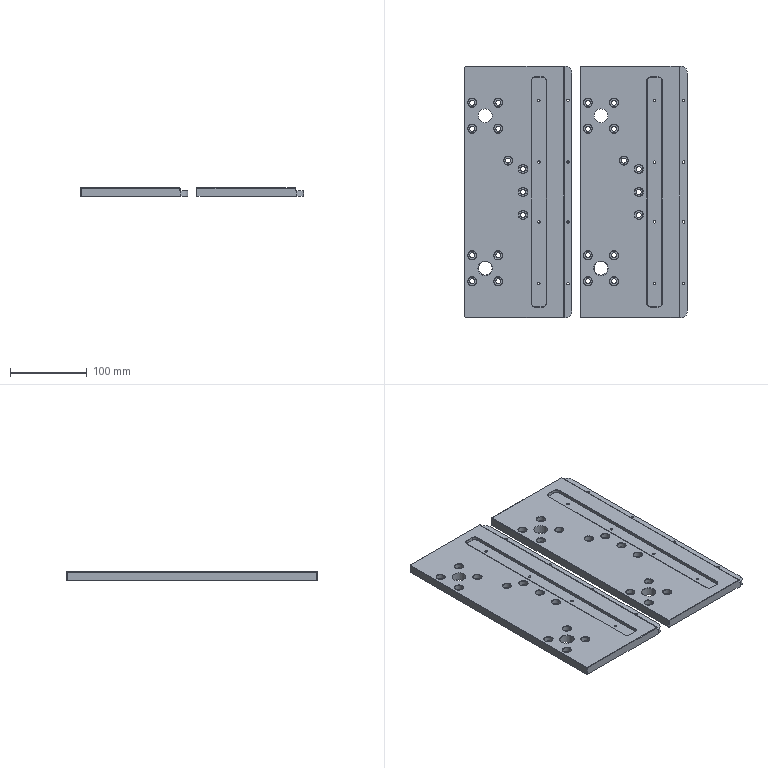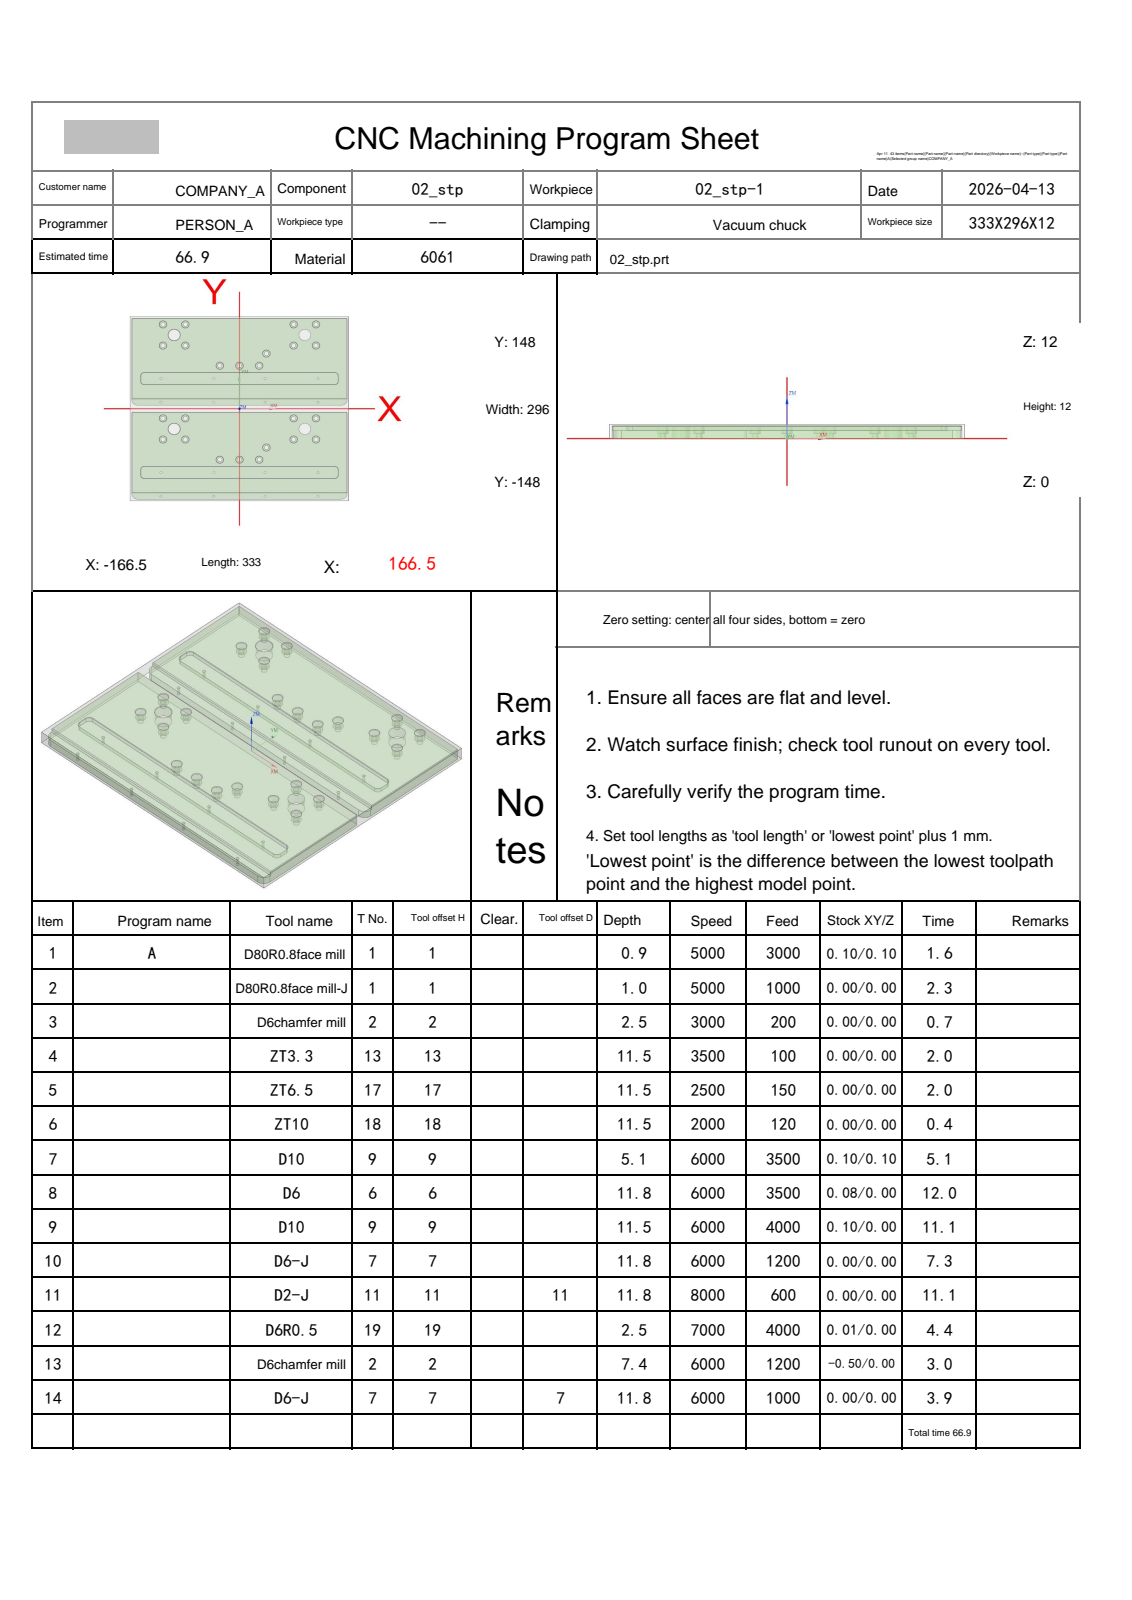NC program | NX | posted by the shop | part box 291 x 328 x 11 mm
Lines 1 to 615 of 9762:
%
O0001
(Machine time: 69.04 MIN)
(===Total Tool:10===)
(T1=D80R0.8 face mill D=80.  R=0.8  D-  H01 Z=11.   )
(T2=D6 chamfer mill   D=6.   R=0.   D-  H02 Z=4.65  )
(T13=ZT3.3  D=3.3  DR_a=118 D-  H13 Z=0.5   )
(T17=ZT6.5  D=6.5  DR_a=118 D-  H17 Z=0.5   )
(T18=ZT10   D=10.  DR_a=118 D-  H18 Z=0.5   )
(T9=D10     D=10.  R=0.   D-  H09 Z=0.5   )
(T6=D6      D=6.   R=0.   D6  H06 Z=0.2   )
(T7=D6-J    D=6.   R=0.   D7  H07 Z=0.2   )
(T11=D2-J   D=2.   R=0.   D11 H11 Z=0.2   )
(T19=D6R0.5 D=6.   R=0.5  D-  H19 Z=9.5   )
G80 G90 G17 G49 G40
G91 G28 Z0
M01
N1 T01 M06
(D80R0.8 face mill  D=80. R=0.8 H=01 ce=0.10 di=0.10)
G00 G90 G54 X-216.097 Y120.945 M03 S5000
G43 H01 Z31.
M08
Z13.55
G01 Z11.55 F3000.
X-204.097 Y121.092
X196.813 Y126.004
X196.897
G02 X204.097 Y118.808 I0.0 J-7.2
G01 Y74.06
G02 X196.199 Y66.065 I-8. J.004
G01 X-196.199 Y61.257
G03 X-204.097 Y53.262 I.102 J-7.999
G01 Y8.514
G03 X-196.897 Y1.317 I7.2 J.004
G01 X-196.813 Y1.318
X196.813 Y6.14
X196.897 Y6.141
G02 X204.097 Y-1.055 I0.0 J-7.2
G01 Y-6.5
Y-45.803
G02 X196.199 Y-53.799 I-8. J.004
G01 X-196.199 Y-58.606
G03 X-204.097 Y-66.602 I.102 J-7.999
G01 Y-111.349
G03 X-196.897 Y-118.546 I7.2 J.004
G01 X-196.813 Y-118.545
X204.097 Y-113.633
X216.097 Y-113.486
Z13.55
G00 X-216.097 Y120.945
Z13.1
G01 Z11.1
X-204.097 Y121.092
X196.813 Y126.004
X196.897
G02 X204.097 Y118.808 I0.0 J-7.2
G01 Y74.06
G02 X196.199 Y66.065 I-8. J.004
G01 X-196.199 Y61.257
G03 X-204.097 Y53.262 I.102 J-7.999
G01 Y8.514
G03 X-196.897 Y1.317 I7.2 J.004
G01 X-196.813 Y1.318
X196.813 Y6.14
X196.897 Y6.141
G02 X204.097 Y-1.055 I0.0 J-7.2
G01 Y-6.5
Y-45.803
G02 X196.199 Y-53.799 I-8. J.004
G01 X-196.199 Y-58.606
G03 X-204.097 Y-66.602 I.102 J-7.999
G01 Y-111.349
G03 X-196.897 Y-118.546 I7.2 J.004
G01 X-196.813 Y-118.545
X204.097 Y-113.633
X216.097 Y-113.486
Z13.1
G00 Z31.
G91 G28 Z0.0
M05
M09
G91 G28 Z0.0
M01
N2 T01 M06
(D80R0.8 face mill-J  D=80. R=0.8 H=01 ce=0.00 di=0.00)
G00 G90 G54 X-215.999 Y120.847 M03 S5000
G43 H01 Z31.
M08
Z13.
G01 Z11. F1000.
X-203.999 Y120.994
X196.714 Y125.909
X196.799
G02 X203.999 Y118.713 I0.0 J-7.2
G01 Y74.013
G02 X196.101 Y66.018 I-8. J.004
G01 X-196.101 Y61.208
G03 X-203.999 Y53.212 I.102 J-7.999
G01 Y8.512
G03 X-196.799 Y1.316 I7.2 J.004
G01 X-196.714 Y1.317
X196.714 Y6.141
X196.799 Y6.142
G02 X203.999 Y-1.054 I0.0 J-7.2
G01 Y-45.755
G02 X196.102 Y-53.75 I-8. J.004
G01 X-196.101 Y-58.56
G03 X-203.999 Y-66.555 I.102 J-7.999
G01 Y-111.255
G03 X-196.799 Y-118.451 I7.2 J.004
G01 X-196.715
X203.999 Y-113.536
X215.999 Y-113.389
Z13.
G00 Z31.
G91 G28 Z0.0
M05
M09
G91 G28 Z0.0
M01
N3 T02 M06
(D6 chamfer mill  D=6. R=0. H=02 ce=0.00 di=0.00)
G00 G90 G54 X39. Y-140.5 M03 S3000
G43 H02 Z31.
M08
G98 G81 X39. Y-140.5 Z9.5 R12. F200.
Y-102.5
X30.05 Y-81.9
X41. Y-62.4
X.05 Y-81.9
X-29.95
X-39. Y-102.5
Y-140.5
X-119.6
Y-102.5
X-116.5 Y-49.5
X-82.5
X-99.5 Y-32.5
X-82.5 Y-15.5
X-116.5
X-119.6 Y10.5
Y48.5
X-116.5 Y101.5
Y135.5
X-99.5 Y118.5
X-82.5 Y135.5
Y101.5
X-29.95 Y69.1
X.05
X-39. Y48.5
Y10.5
X39.
Y48.5
X30.05 Y69.1
X41. Y88.6
X82.5 Y101.5
Y135.5
X116.5
X99.5 Y118.5
X116.5 Y101.5
X119.6 Y48.5
Y10.5
X116.5 Y-15.5
X82.5
X99.5 Y-32.5
X82.5 Y-49.5
X116.5
X119.6 Y-102.5
Y-140.5
G80
G00 Z31.
G91 G28 Z0.0
M05
M09
G91 G28 Z0.0
M01
N4 T13 M06
(ZT3.3 D=3.3 DR_a=118 H=13)
G00 G90 G54 X-119.6 Y-102.5 M03 S3500
G43 H13 Z31.
M08
G98 G83 X-119.6 Y-102.5 Z.5 R12. F100. Q1.5
Y-140.5
X-39.
Y-102.5
X39.
Y-140.5
X119.6
Y-102.5
Y10.5
Y48.5
X39.
Y10.5
X-39.
Y48.5
X-119.6
Y10.5
G80
G00 Z31.
G91 G28 Z0.0
M05
M09
G91 G28 Z0.0
M01
N5 T17 M06
(ZT6.5 D=6.5 DR_a=118 H=17)
G00 G90 G54 X-82.5 Y-15.5 M03 S2500
G43 H17 Z31.
M08
G98 G83 X-82.5 Y-15.5 Z.5 R12. F150. Q3.
X-116.5
Y-49.5
X-82.5
X-29.95 Y-81.9
X.05
X30.05
X41. Y-62.4
X82.5 Y-49.5
X116.5
Y-15.5
X82.5
X116.5 Y101.5
Y135.5
X82.5
Y101.5
X41. Y88.6
X30.05 Y69.1
X.05
X-29.95
X-82.5 Y101.5
Y135.5
X-116.5
Y101.5
G80
G00 Z31.
G91 G28 Z0.0
M05
M09
G91 G28 Z0.0
M01
N6 T18 M06
(ZT10 D=10. DR_a=118 H=18)
G00 G90 G54 X99.5 Y118.5 M03 S2000
G43 H18 Z31.
M08
G98 G83 X99.5 Y118.5 Z.5 R12. F120. Q1.5
Y-32.5
X-99.5
Y118.5
G80
G00 Z31.
G91 G28 Z0.0
M05
M09
G91 G28 Z0.0
M01
N7 T09 M06
(D10  D=10. R=0. H=09 ce=0.10 di=0.10)
G00 G90 G54 X140.478 Y42.523 M03 S6000
G43 H09 Z31.
M08
Z12.036
G01 Z11.536 F3500.
X141.001 Y48.5
Y49.001
X-141.001
Y47.999
X141.001
Y48.5
X145.501
Y53.
G03 X145. Y53.501 I-.501 J0.0
G01 X-145.
G03 X-145.501 Y53. I0.0 J-.501
G01 Y44.
G03 X-145. Y43.499 I.501 J0.0
G01 X145.
G03 X145.501 Y44. I0.0 J.501
G01 Y48.5
Z12.536
G00 Z13.
X27.595 Y48.681
Z12.036
M03 S6000
G01 X0.0 Z11.073 F2800.
Y48.981
M03 S6000
X-140.981 F3500.
Y48.019
X140.981
Y48.981
X0.0
Y53.481
X-145.
G03 X-145.481 Y53. I0.0 J-.481
G01 Y44.
G03 X-145. Y43.519 I.481 J0.0
G01 X145.
G03 X145.481 Y44. I0.0 J.481
G01 Y53.
G03 X145. Y53.481 I-.481 J0.0
G01 X0.0
Z12.073
G00 Z12.536
X27.595 Y48.518
Z11.573
M03 S6000
G01 X0.0 Z10.609 F2800.
M03 S6000
X-140.518 F3500.
Y48.482
X140.518
Y48.518
X0.0
Y53.018
X-145.
X-145.019 Y53.019
X-145.018 Y53.
Y44.
X-145.019 Y43.981
X-145. Y43.982
X145.
X145.019 Y43.981
X145.018 Y44.
Y53.
X145.019 Y53.019
X145. Y53.018
X0.0
Z11.609
G00 Z12.073
X27.595 Y52.65
Z11.109
M03 S6000
G01 X0.0 Z10.145 F2800.
Y52.95
M03 S6000
X-144.95 F3500.
Y44.05
X144.95
Y52.95
X0.0
Z11.145
G00 Z11.609
X27.595 Y52.65
Z10.645
M03 S6000
G01 X0.0 Z9.682 F2800.
Y52.95
M03 S6000
X-144.95 F3500.
Y44.05
X144.95
Y52.95
X0.0
Z10.682
G00 Z11.145
X27.595 Y52.65
Z10.182
M03 S6000
G01 X0.0 Z9.218 F2800.
Y52.95
M03 S6000
X-144.95 F3500.
Y44.05
X144.95
Y52.95
X0.0
Z10.218
G00 Z10.682
X27.595 Y52.65
Z9.718
M03 S6000
G01 X0.0 Z8.755 F2800.
Y52.95
M03 S6000
X-144.95 F3500.
Y44.05
X144.95
Y52.95
X0.0
Z9.755
G00 Z10.218
X27.595 Y52.65
Z9.255
M03 S6000
G01 X0.0 Z8.291 F2800.
Y52.95
M03 S6000
X-144.95 F3500.
Y44.05
X144.95
Y52.95
X0.0
Z9.291
G00 Z9.755
X27.595 Y52.65
Z8.791
M03 S6000
G01 X0.0 Z7.827 F2800.
Y52.95
M03 S6000
X-144.95 F3500.
Y44.05
X144.95
Y52.95
X0.0
Z8.827
G00 Z9.291
X27.595 Y52.65
Z8.327
M03 S6000
G01 X0.0 Z7.364 F2800.
Y52.95
M03 S6000
X-144.95 F3500.
Y44.05
X144.95
Y52.95
X0.0
Z8.364
G00 Z8.827
X27.595 Y52.65
Z7.864
M03 S6000
G01 X0.0 Z6.9 F2800.
Y52.95
M03 S6000
X-144.95 F3500.
Y44.05
X144.95
Y52.95
X0.0
Z7.9
G00 Z31.
X140.478 Y-108.477
Z12.036
G01 Z11.536
X141.001 Y-102.5
Y-101.999
X-141.001
Y-103.001
X141.001
Y-102.5
X145.501
Y-98.
G03 X145. Y-97.499 I-.501 J0.0
G01 X-145.
G03 X-145.501 Y-98. I0.0 J-.501
G01 Y-107.
G03 X-145. Y-107.501 I.501 J0.0
G01 X145.
G03 X145.501 Y-107. I0.0 J.501
G01 Y-102.5
Z12.536
G00 Z13.
X-27.595 Y-102.681
Z12.036
M03 S6000
G01 X0.0 Z11.073 F2800.
Y-102.981
M03 S6000
X140.981 F3500.
Y-102.019
X-140.981
Y-102.981
X0.0
Y-107.481
X145.
G03 X145.481 Y-107. I0.0 J.481
G01 Y-98.
G03 X145. Y-97.519 I-.481 J0.0
G01 X-145.
G03 X-145.481 Y-98. I0.0 J-.481
G01 Y-107.
G03 X-145. Y-107.481 I.481 J0.0
G01 X0.0
Z12.073
G00 Z12.536
X-27.595 Y-102.518
Z11.573
M03 S6000
G01 X0.0 Z10.609 F2800.
M03 S6000
X140.518 F3500.
Y-102.482
X-140.518
Y-102.518
X0.0
Y-107.018
X145.
X145.019 Y-107.019
X145.018 Y-107.
Y-98.
X145.019 Y-97.981
X145. Y-97.982
X-145.
X-145.019 Y-97.981
X-145.018 Y-98.
Y-107.
X-145.019 Y-107.019
X-145. Y-107.018
X0.0
Z11.609
G00 Z12.073
X-27.595 Y-106.65
Z11.109
M03 S6000
G01 X0.0 Z10.145 F2800.
Y-106.95
M03 S6000
X144.95 F3500.
Y-98.05
X-144.95
Y-106.95
X0.0
Z11.145
G00 Z11.609
X-27.595 Y-106.65
Z10.645
M03 S6000
G01 X0.0 Z9.682 F2800.
Y-106.95
M03 S6000
X144.95 F3500.
Y-98.05
X-144.95
Y-106.95
X0.0
Z10.682
G00 Z11.145
X-27.595 Y-106.65
Z10.182
M03 S6000
G01 X0.0 Z9.218 F2800.
Y-106.95
M03 S6000
X144.95 F3500.
Y-98.05
X-144.95
Y-106.95
X0.0
Z10.218
G00 Z10.682
X-27.595 Y-106.65
Z9.718
M03 S6000
G01 X0.0 Z8.755 F2800.
Y-106.95
M03 S6000
X144.95 F3500.
Y-98.05
X-144.95
Y-106.95
X0.0
Z9.755
G00 Z10.218
X-27.595 Y-106.65
Z9.255
M03 S6000
G01 X0.0 Z8.291 F2800.
Y-106.95
M03 S6000
X144.95 F3500.
Y-98.05
X-144.95
Y-106.95
X0.0
Z9.291
G00 Z9.755
X-27.595 Y-106.65
Z8.791
M03 S6000
G01 X0.0 Z7.827 F2800.
Y-106.95
M03 S6000
X144.95 F3500.
Y-98.05
X-144.95
Y-106.95
X0.0
Z8.827
G00 Z9.291
X-27.595 Y-106.65
Z8.327
M03 S6000
G01 X0.0 Z7.364 F2800.
Y-106.95
M03 S6000
X144.95 F3500.
Y-98.05
X-144.95
Y-106.95
X0.0
Z8.364
G00 Z8.827
X-27.595 Y-106.65
Z7.864
M03 S6000
G01 X0.0 Z6.9 F2800.
Y-106.95
M03 S6000
X144.95 F3500.
Y-98.05
X-144.95
Y-106.95
X0.0
Z7.9
G00 Z31.
G91 G28 Z0.0
M05
M09
G91 G28 Z0.0
M01